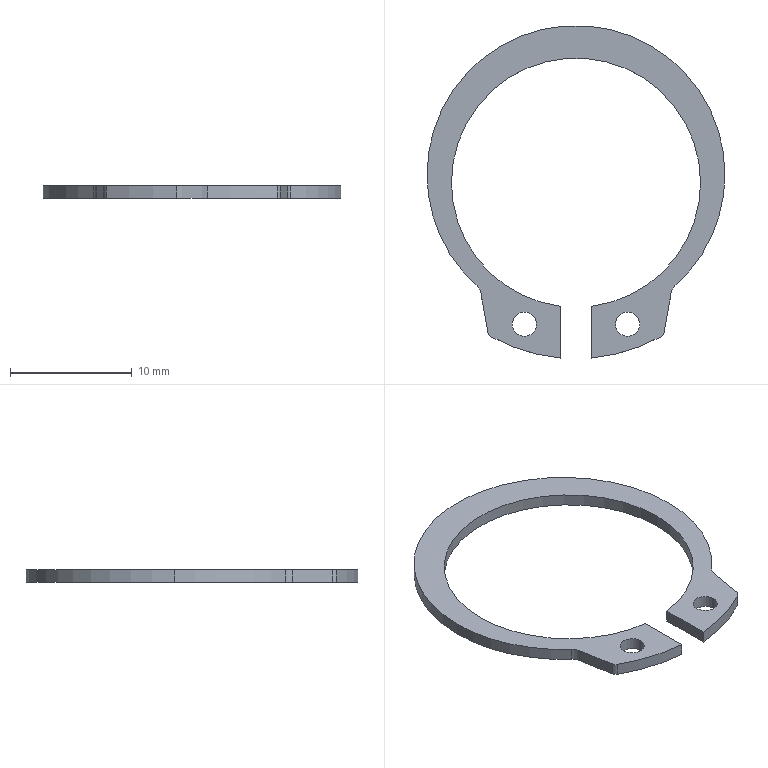Part | STEP file | 1 solid | 22 faces | box 24.52 x 27.353 x 1 mm | volume 170.96 mm3 | cylinder 16 | plane 6 | commonest cylinder face diameters 2 x6 20.5 x3 24.52 x3 1 x2 28.955 x2